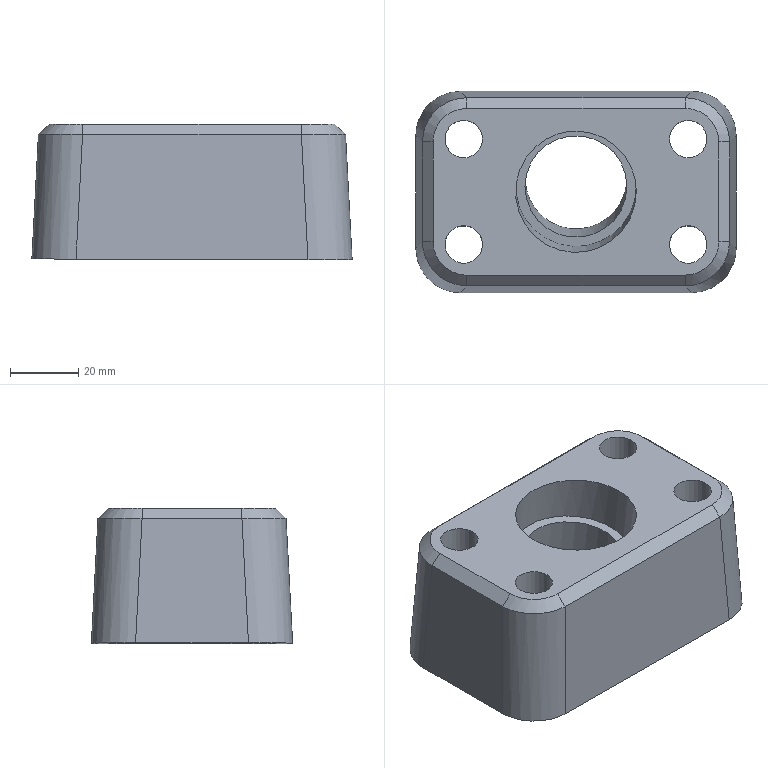Part | STEP file | solid 244 | 1 solid | 33 faces | box 94.183 x 59.188 x 39.916 mm | volume 147837 mm3 | plane 14 | cylinder 14 | spline 4 | other 1 | commonest cylinder face diameters 11 x4 18 x4 26 x4 30 x1 35.5 x1